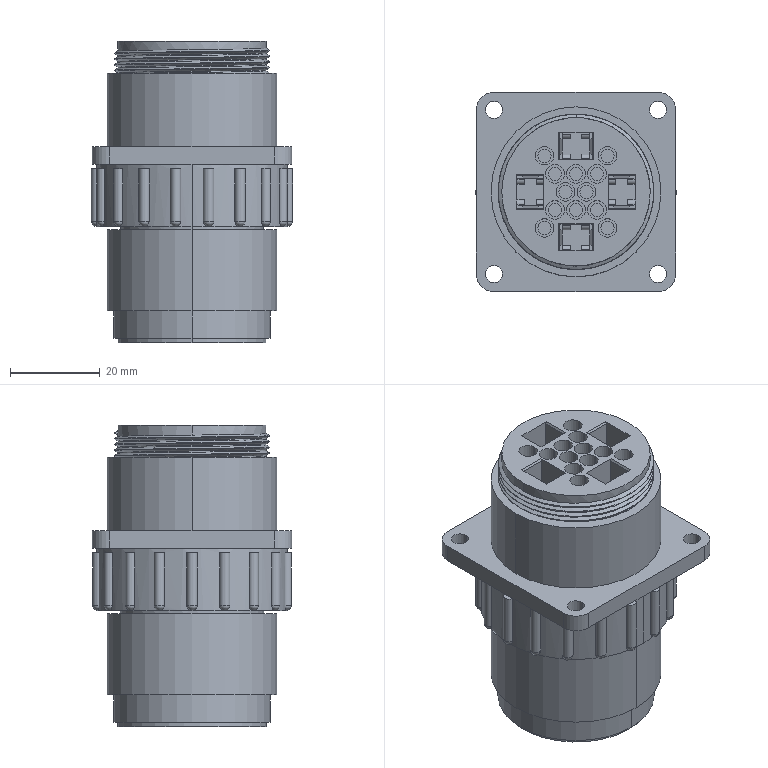Part | STEP file | _AMP_ASM.stp.STEP | 1 solid | 542 faces | box 44.856 x 44.45 x 67.183 mm | volume 70533 mm3 | plane 317 | cylinder 188 | sphere 18 | spline 11 | cone 8 | commonest cylinder face diameters 4.14 x48 2.934 x24 2.388 x18 2.032 x16 36.525 x13 33.071 x12